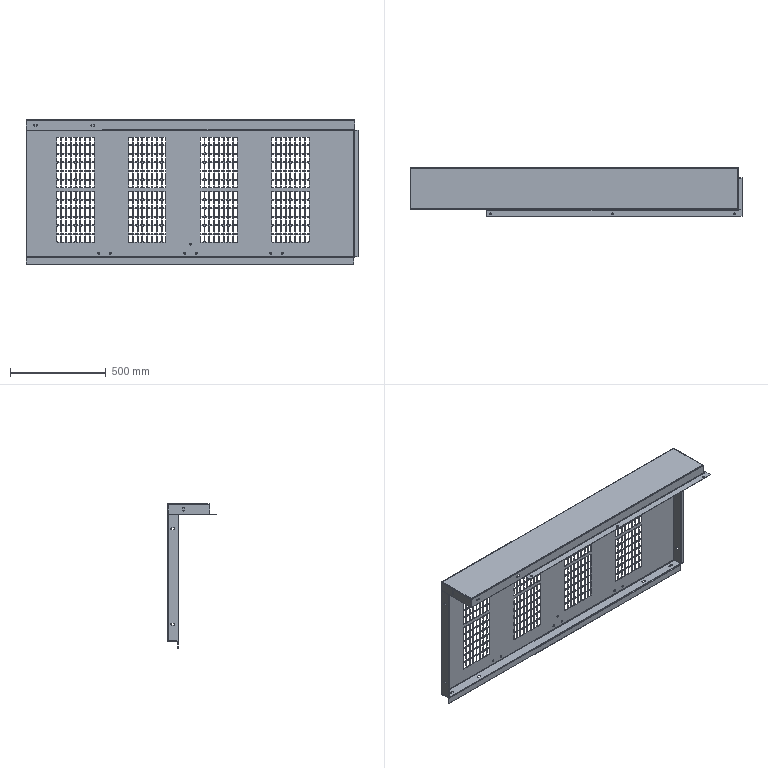Part | STEP file | SYL_0392D6J1SYL0380DJ100-567986 | 1 solid | 3275 faces | volume 3380150 mm3 | plane 1653 | cylinder 1610 | spline 12 | commonest cylinder face diameters 5 x1536 10 x34 10.5 x18 4 x11 8 x11